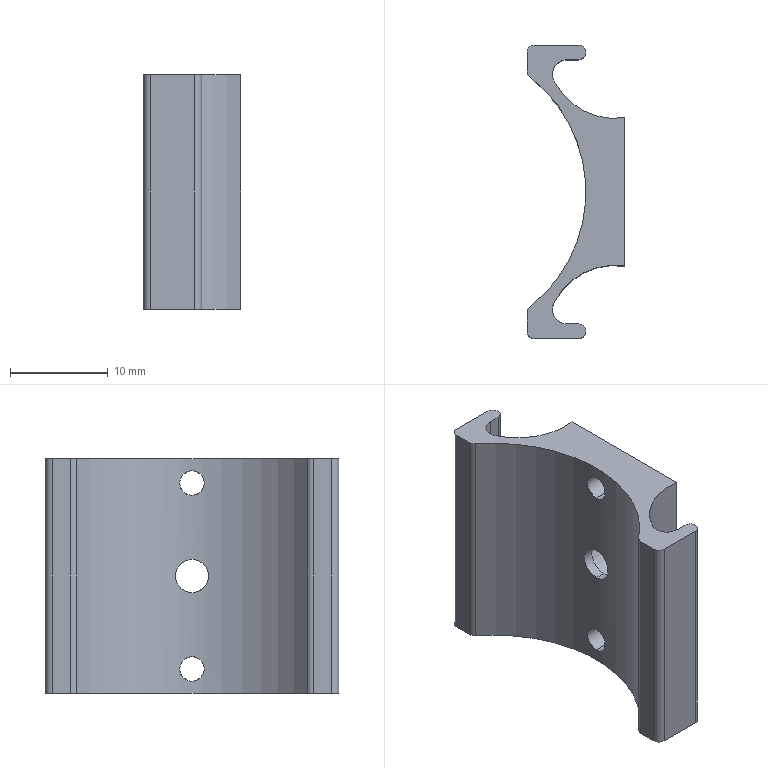Part | SolidWorks | features HoleWzd 2, Extrusion 1 | 1 solid | 31 faces | box 10 x 30 x 24 mm | volume 2596 mm3 | cylinder 21 | plane 10 | commonest cylinder face diameters 1.5 x6 2.5 x4 3 x4 3.4 x2 6 x2 14 x2
STEP:
#1=CARTESIAN_POINT('',(2.5,0.,3.));
#2=VERTEX_POINT('',#1);
#3=CARTESIAN_POINT('',(2.5,0.,-3.));
#4=VERTEX_POINT('',#3);
#5=CARTESIAN_POINT('',(2.5,0.,0.));
#6=DIRECTION('',(1.,0.,0.));
#7=DIRECTION('',(0.,0.,-1.));
#8=AXIS2_PLACEMENT_3D('',#5,#6,#7);
#9=CIRCLE('',#8,3.);
#10=EDGE_CURVE('',#2,#4,#9,.T.);
#11=ORIENTED_EDGE('',*,*,#10,.F.);
#12=CARTESIAN_POINT('',(5.5,0.,3.));
#13=VERTEX_POINT('',#12);
#14=CARTESIAN_POINT('',(5.5,0.,3.));
#15=DIRECTION('',(1.,0.,0.));
#16=VECTOR('',#15,1000.);
#17=LINE('',#14,#16);
#18=EDGE_CURVE('',#2,#13,#17,.T.);
#19=ORIENTED_EDGE('',*,*,#18,.T.);
#20=CARTESIAN_POINT('',(5.5,0.,-3.));
#21=VERTEX_POINT('',#20);
#22=CARTESIAN_POINT('',(5.5,0.,0.));
#23=DIRECTION('',(1.,0.,0.));
#24=DIRECTION('',(0.,0.,-1.));
#25=AXIS2_PLACEMENT_3D('',#22,#23,#24);
#26=CIRCLE('',#25,3.);
#27=EDGE_CURVE('',#13,#21,#26,.T.);
#28=ORIENTED_EDGE('',*,*,#27,.T.);
#29=CARTESIAN_POINT('',(5.5,0.,-3.));
#30=DIRECTION('',(1.,0.,0.));
#31=VECTOR('',#30,1000.);
#32=LINE('',#29,#31);
#33=EDGE_CURVE('',#4,#21,#32,.T.);
#34=ORIENTED_EDGE('',*,*,#33,.F.);
#35=EDGE_LOOP('',(#11,#19,#28,#34));
#36=FACE_OUTER_BOUND('',#35,.T.);
#37=CARTESIAN_POINT('',(5.5,0.,0.));
#38=DIRECTION('',(1.,0.,0.));
#39=DIRECTION('',(0.,0.,-1.));
#40=AXIS2_PLACEMENT_3D('',#37,#38,#39);
#41=CYLINDRICAL_SURFACE('',#40,3.);
#42=ADVANCED_FACE('',(#36),#41,.F.);
#43=CARTESIAN_POINT('',(1.5,0.,1.7));
#44=VERTEX_POINT('',#43);
#45=CARTESIAN_POINT('',(1.5,0.,-1.7));
#46=VERTEX_POINT('',#45);
#47=CARTESIAN_POINT('',(1.5,0.,1.7));
#48=CARTESIAN_POINT('',(1.5,-0.2219,1.7));
#49=CARTESIAN_POINT('',(1.495,-0.4457,1.655));
#50=CARTESIAN_POINT('',(1.477,-0.8549,1.486));
#51=CARTESIAN_POINT('',(1.464,-1.044,1.359));
#52=CARTESIAN_POINT('',(1.446,-1.28,1.125));
#53=CARTESIAN_POINT('',(1.439,-1.351,1.037));
#54=CARTESIAN_POINT('',(1.427,-1.475,0.8527));
#55=CARTESIAN_POINT('',(1.422,-1.527,0.7551));
#56=CARTESIAN_POINT('',(1.413,-1.613,0.5494));
#57=CARTESIAN_POINT('',(1.409,-1.645,0.4414));
#58=CARTESIAN_POINT('',(1.405,-1.689,0.2241));
#59=CARTESIAN_POINT('',(1.403,-1.7,0.1136));
#60=CARTESIAN_POINT('',(1.403,-1.7,-0.1111));
#61=CARTESIAN_POINT('',(1.405,-1.689,-0.2217));
#62=CARTESIAN_POINT('',(1.409,-1.646,-0.4391));
#63=CARTESIAN_POINT('',(1.413,-1.613,-0.5471));
#64=CARTESIAN_POINT('',(1.422,-1.528,-0.753));
#65=CARTESIAN_POINT('',(1.427,-1.476,-0.8506));
#66=CARTESIAN_POINT('',(1.439,-1.353,-1.035));
#67=CARTESIAN_POINT('',(1.445,-1.281,-1.123));
#68=CARTESIAN_POINT('',(1.464,-1.046,-1.358));
#69=CARTESIAN_POINT('',(1.477,-0.857,-1.485));
#70=CARTESIAN_POINT('',(1.495,-0.4481,-1.655));
#71=CARTESIAN_POINT('',(1.5,-0.2248,-1.7));
#72=CARTESIAN_POINT('',(1.5,0.,-1.7));
#73=B_SPLINE_CURVE_WITH_KNOTS('',3,(#47,#48,#49,#50,#51,#52,#53,#54,#55,#56,#57,#58,#59,#60,#61,#62,#63,#64,#65,#66,#67,#68,#69,#70,#71,#72),.UNSPECIFIED.,.F.,.F.,(4,2,2,2,2,2,2,2,2,2,2,2,4),(0.005319,0.005984,0.006649,0.006981,0.007313,0.007646,0.007978,0.008311,0.008643,0.008975,0.009308,0.009972,0.01064),.UNSPECIFIED.);
#74=EDGE_CURVE('',#44,#46,#73,.T.);
#75=ORIENTED_EDGE('',*,*,#74,.F.);
#76=CARTESIAN_POINT('',(2.5,0.,1.7));
#77=VERTEX_POINT('',#76);
#78=CARTESIAN_POINT('',(5.5,0.,1.7));
#79=DIRECTION('',(1.,0.,0.));
#80=VECTOR('',#79,1000.);
#81=LINE('',#78,#80);
#82=EDGE_CURVE('',#44,#77,#81,.T.);
#83=ORIENTED_EDGE('',*,*,#82,.T.);
#84=CARTESIAN_POINT('',(2.5,0.,-1.7));
#85=VERTEX_POINT('',#84);
#86=CARTESIAN_POINT('',(2.5,0.,0.));
#87=DIRECTION('',(1.,0.,0.));
#88=DIRECTION('',(0.,0.,-1.));
#89=AXIS2_PLACEMENT_3D('',#86,#87,#88);
#90=CIRCLE('',#89,1.7);
#91=EDGE_CURVE('',#77,#85,#90,.T.);
#92=ORIENTED_EDGE('',*,*,#91,.T.);
#93=CARTESIAN_POINT('',(5.5,0.,-1.7));
#94=DIRECTION('',(1.,0.,0.));
#95=VECTOR('',#94,1000.);
#96=LINE('',#93,#95);
#97=EDGE_CURVE('',#46,#85,#96,.T.);
#98=ORIENTED_EDGE('',*,*,#97,.F.);
#99=EDGE_LOOP('',(#75,#83,#92,#98));
#100=FACE_OUTER_BOUND('',#99,.T.);
#101=CARTESIAN_POINT('',(5.5,0.,0.));
#102=DIRECTION('',(1.,0.,0.));
#103=DIRECTION('',(0.,0.,-1.));
#104=AXIS2_PLACEMENT_3D('',#101,#102,#103);
#105=CYLINDRICAL_SURFACE('',#104,1.7);
#106=ADVANCED_FACE('',(#100),#105,.F.);
#107=CARTESIAN_POINT('',(1.5,0.,10.75));
#108=VERTEX_POINT('',#107);
#109=CARTESIAN_POINT('',(1.5,0.,8.25));
#110=VERTEX_POINT('',#109);
#111=CARTESIAN_POINT('',(1.5,0.,10.75));
#112=CARTESIAN_POINT('',(1.5,-0.1632,10.75));
#113=CARTESIAN_POINT('',(1.497,-0.3276,10.717));
#114=CARTESIAN_POINT('',(1.488,-0.6285,10.593));
#115=CARTESIAN_POINT('',(1.481,-0.768,10.5));
#116=CARTESIAN_POINT('',(1.467,-0.9986,10.269));
#117=CARTESIAN_POINT('',(1.46,-1.092,10.131));
#118=CARTESIAN_POINT('',(1.451,-1.217,9.828));
#119=CARTESIAN_POINT('',(1.448,-1.25,9.666));
#120=CARTESIAN_POINT('',(1.448,-1.25,9.336));
#121=CARTESIAN_POINT('',(1.451,-1.218,9.174));
#122=CARTESIAN_POINT('',(1.458,-1.124,8.946));
#123=CARTESIAN_POINT('',(1.461,-1.085,8.875));
#124=CARTESIAN_POINT('',(1.467,-0.9948,8.739));
#125=CARTESIAN_POINT('',(1.47,-0.9421,8.674));
#126=CARTESIAN_POINT('',(1.481,-0.7693,8.501));
#127=CARTESIAN_POINT('',(1.488,-0.63,8.408));
#128=CARTESIAN_POINT('',(1.497,-0.3294,8.283));
#129=CARTESIAN_POINT('',(1.5,-0.1652,8.25));
#130=CARTESIAN_POINT('',(1.5,0.,8.25));
#131=B_SPLINE_CURVE_WITH_KNOTS('',3,(#111,#112,#113,#114,#115,#116,#117,#118,#119,#120,#121,#122,#123,#124,#125,#126,#127,#128,#129,#130),.UNSPECIFIED.,.F.,.F.,(4,2,2,2,2,2,2,2,2,4),(0.00391,0.004398,0.004887,0.005376,0.005864,0.006353,0.006597,0.006841,0.00733,0.007819),.UNSPECIFIED.);
#132=EDGE_CURVE('',#108,#110,#131,.T.);
#133=ORIENTED_EDGE('',*,*,#132,.F.);
#134=CARTESIAN_POINT('',(5.5,0.,10.75));
#135=VERTEX_POINT('',#134);
#136=CARTESIAN_POINT('',(5.5,0.,10.75));
#137=DIRECTION('',(1.,0.,0.));
#138=VECTOR('',#137,1000.);
#139=LINE('',#136,#138);
#140=EDGE_CURVE('',#108,#135,#139,.T.);
#141=ORIENTED_EDGE('',*,*,#140,.T.);
#142=CARTESIAN_POINT('',(5.5,0.,8.25));
#143=VERTEX_POINT('',#142);
#144=CARTESIAN_POINT('',(5.5,0.,9.5));
#145=DIRECTION('',(1.,0.,0.));
#146=DIRECTION('',(0.,0.,-1.));
#147=AXIS2_PLACEMENT_3D('',#144,#145,#146);
#148=CIRCLE('',#147,1.25);
#149=EDGE_CURVE('',#135,#143,#148,.T.);
#150=ORIENTED_EDGE('',*,*,#149,.T.);
#151=CARTESIAN_POINT('',(5.5,0.,8.25));
#152=DIRECTION('',(1.,0.,0.));
#153=VECTOR('',#152,1000.);
#154=LINE('',#151,#153);
#155=EDGE_CURVE('',#110,#143,#154,.T.);
#156=ORIENTED_EDGE('',*,*,#155,.F.);
#157=EDGE_LOOP('',(#133,#141,#150,#156));
#158=FACE_OUTER_BOUND('',#157,.T.);
#159=CARTESIAN_POINT('',(5.5,0.,9.5));
#160=DIRECTION('',(1.,0.,0.));
#161=DIRECTION('',(0.,0.,-1.));
#162=AXIS2_PLACEMENT_3D('',#159,#160,#161);
#163=CYLINDRICAL_SURFACE('',#162,1.25);
#164=ADVANCED_FACE('',(#158),#163,.F.);
#165=CARTESIAN_POINT('',(1.5,0.,-8.25));
#166=VERTEX_POINT('',#165);
#167=CARTESIAN_POINT('',(1.5,0.,-10.75));
#168=VERTEX_POINT('',#167);
#169=CARTESIAN_POINT('',(1.5,0.,-8.25));
#170=CARTESIAN_POINT('',(1.5,-0.1632,-8.25));
#171=CARTESIAN_POINT('',(1.497,-0.3276,-8.283));
#172=CARTESIAN_POINT('',(1.488,-0.6285,-8.407));
#173=CARTESIAN_POINT('',(1.481,-0.768,-8.5));
#174=CARTESIAN_POINT('',(1.467,-0.9986,-8.731));
#175=CARTESIAN_POINT('',(1.46,-1.092,-8.869));
#176=CARTESIAN_POINT('',(1.451,-1.217,-9.172));
#177=CARTESIAN_POINT('',(1.448,-1.25,-9.334));
#178=CARTESIAN_POINT('',(1.448,-1.25,-9.664));
#179=CARTESIAN_POINT('',(1.451,-1.218,-9.826));
#180=CARTESIAN_POINT('',(1.458,-1.124,-10.054));
#181=CARTESIAN_POINT('',(1.461,-1.085,-10.125));
#182=CARTESIAN_POINT('',(1.467,-0.9948,-10.261));
#183=CARTESIAN_POINT('',(1.47,-0.9421,-10.326));
#184=CARTESIAN_POINT('',(1.481,-0.7693,-10.499));
#185=CARTESIAN_POINT('',(1.488,-0.63,-10.592));
#186=CARTESIAN_POINT('',(1.497,-0.3294,-10.717));
#187=CARTESIAN_POINT('',(1.5,-0.1652,-10.75));
#188=CARTESIAN_POINT('',(1.5,0.,-10.75));
#189=B_SPLINE_CURVE_WITH_KNOTS('',3,(#169,#170,#171,#172,#173,#174,#175,#176,#177,#178,#179,#180,#181,#182,#183,#184,#185,#186,#187,#188),.UNSPECIFIED.,.F.,.F.,(4,2,2,2,2,2,2,2,2,4),(0.00391,0.004398,0.004887,0.005376,0.005864,0.006353,0.006597,0.006841,0.00733,0.007819),.UNSPECIFIED.);
#190=EDGE_CURVE('',#166,#168,#189,.T.);
#191=ORIENTED_EDGE('',*,*,#190,.F.);
#192=CARTESIAN_POINT('',(5.5,0.,-8.25));
#193=VERTEX_POINT('',#192);
#194=CARTESIAN_POINT('',(5.5,0.,-8.25));
#195=DIRECTION('',(1.,0.,0.));
#196=VECTOR('',#195,1000.);
#197=LINE('',#194,#196);
#198=EDGE_CURVE('',#166,#193,#197,.T.);
#199=ORIENTED_EDGE('',*,*,#198,.T.);
#200=CARTESIAN_POINT('',(5.5,0.,-10.75));
#201=VERTEX_POINT('',#200);
#202=CARTESIAN_POINT('',(5.5,0.,-9.5));
#203=DIRECTION('',(1.,0.,0.));
#204=DIRECTION('',(0.,0.,-1.));
#205=AXIS2_PLACEMENT_3D('',#202,#203,#204);
#206=CIRCLE('',#205,1.25);
#207=EDGE_CURVE('',#193,#201,#206,.T.);
#208=ORIENTED_EDGE('',*,*,#207,.T.);
#209=CARTESIAN_POINT('',(5.5,0.,-10.75));
#210=DIRECTION('',(1.,0.,0.));
#211=VECTOR('',#210,1000.);
#212=LINE('',#209,#211);
#213=EDGE_CURVE('',#168,#201,#212,.T.);
#214=ORIENTED_EDGE('',*,*,#213,.F.);
#215=EDGE_LOOP('',(#191,#199,#208,#214));
#216=FACE_OUTER_BOUND('',#215,.T.);
#217=CARTESIAN_POINT('',(5.5,0.,-9.5));
#218=DIRECTION('',(1.,0.,0.));
#219=DIRECTION('',(0.,0.,-1.));
#220=AXIS2_PLACEMENT_3D('',#217,#218,#219);
#221=CYLINDRICAL_SURFACE('',#220,1.25);
#222=ADVANCED_FACE('',(#216),#221,.F.);
#223=CARTESIAN_POINT('',(-1.899,-12.,12.));
#224=VERTEX_POINT('',#223);
#225=CARTESIAN_POINT('',(-1.735,-11.318,12.));
#226=VERTEX_POINT('',#225);
#227=CARTESIAN_POINT('',(-0.399,-12.,12.));
#228=DIRECTION('',(0.,0.,-1.));
#229=DIRECTION('',(1.,0.,0.));
#230=AXIS2_PLACEMENT_3D('',#227,#228,#229);
#231=CIRCLE('',#230,1.5);
#232=EDGE_CURVE('',#224,#226,#231,.T.);
#233=ORIENTED_EDGE('',*,*,#232,.F.);
#234=CARTESIAN_POINT('',(-1.899,-12.,-12.));
#235=VERTEX_POINT('',#234);
#236=CARTESIAN_POINT('',(-1.899,-12.,12.));
#237=DIRECTION('',(0.,0.,-1.));
#238=VECTOR('',#237,1000.);
#239=LINE('',#236,#238);
#240=EDGE_CURVE('',#224,#235,#239,.T.);
#241=ORIENTED_EDGE('',*,*,#240,.T.);
#242=CARTESIAN_POINT('',(-1.735,-11.318,-12.));
#243=VERTEX_POINT('',#242);
#244=CARTESIAN_POINT('',(-0.399,-12.,-12.));
#245=DIRECTION('',(0.,0.,-1.));
#246=DIRECTION('',(1.,0.,0.));
#247=AXIS2_PLACEMENT_3D('',#244,#245,#246);
#248=CIRCLE('',#247,1.5);
#249=EDGE_CURVE('',#235,#243,#248,.T.);
#250=ORIENTED_EDGE('',*,*,#249,.T.);
#251=CARTESIAN_POINT('',(-1.735,-11.318,12.));
#252=DIRECTION('',(0.,0.,-1.));
#253=VECTOR('',#252,1000.);
#254=LINE('',#251,#253);
#255=EDGE_CURVE('',#226,#243,#254,.T.);
#256=ORIENTED_EDGE('',*,*,#255,.F.);
#257=EDGE_LOOP('',(#233,#241,#250,#256));
#258=FACE_OUTER_BOUND('',#257,.T.);
#259=CARTESIAN_POINT('',(-0.399,-12.,12.));
#260=DIRECTION('',(0.,0.,-1.));
#261=DIRECTION('',(-1.,0.,0.));
#262=AXIS2_PLACEMENT_3D('',#259,#260,#261);
#263=CYLINDRICAL_SURFACE('',#262,1.5);
#264=ADVANCED_FACE('',(#258),#263,.F.);
#265=CARTESIAN_POINT('',(-1.899,12.,12.));
#266=VERTEX_POINT('',#265);
#267=CARTESIAN_POINT('',(-0.399,13.5,12.));
#268=VERTEX_POINT('',#267);
#269=CARTESIAN_POINT('',(-0.399,12.,12.));
#270=DIRECTION('',(0.,0.,-1.));
#271=DIRECTION('',(1.,0.,0.));
#272=AXIS2_PLACEMENT_3D('',#269,#270,#271);
#273=CIRCLE('',#272,1.5);
#274=EDGE_CURVE('',#266,#268,#273,.T.);
#275=ORIENTED_EDGE('',*,*,#274,.F.);
#276=CARTESIAN_POINT('',(-1.899,12.,-12.));
#277=VERTEX_POINT('',#276);
#278=CARTESIAN_POINT('',(-1.899,12.,12.));
#279=DIRECTION('',(0.,0.,-1.));
#280=VECTOR('',#279,1000.);
#281=LINE('',#278,#280);
#282=EDGE_CURVE('',#266,#277,#281,.T.);
#283=ORIENTED_EDGE('',*,*,#282,.T.);
#284=CARTESIAN_POINT('',(-0.399,13.5,-12.));
#285=VERTEX_POINT('',#284);
#286=CARTESIAN_POINT('',(-0.399,12.,-12.));
#287=DIRECTION('',(0.,0.,-1.));
#288=DIRECTION('',(1.,0.,0.));
#289=AXIS2_PLACEMENT_3D('',#286,#287,#288);
#290=CIRCLE('',#289,1.5);
#291=EDGE_CURVE('',#277,#285,#290,.T.);
#292=ORIENTED_EDGE('',*,*,#291,.T.);
#293=CARTESIAN_POINT('',(-0.399,13.5,12.));
#294=DIRECTION('',(0.,0.,-1.));
#295=VECTOR('',#294,1000.);
#296=LINE('',#293,#295);
#297=EDGE_CURVE('',#268,#285,#296,.T.);
#298=ORIENTED_EDGE('',*,*,#297,.F.);
#299=EDGE_LOOP('',(#275,#283,#292,#298));
#300=FACE_OUTER_BOUND('',#299,.T.);
#301=CARTESIAN_POINT('',(-0.399,12.,12.));
#302=DIRECTION('',(0.,0.,-1.));
#303=DIRECTION('',(-1.,0.,0.));
#304=AXIS2_PLACEMENT_3D('',#301,#302,#303);
#305=CYLINDRICAL_SURFACE('',#304,1.5);
#306=ADVANCED_FACE('',(#300),#305,.F.);
#307=ORIENTED_EDGE('',*,*,#282,.F.);
#308=CARTESIAN_POINT('',(-1.735,11.318,12.));
#309=VERTEX_POINT('',#308);
#310=CARTESIAN_POINT('',(-0.399,12.,12.));
#311=DIRECTION('',(0.,0.,-1.));
#312=DIRECTION('',(1.,0.,0.));
#313=AXIS2_PLACEMENT_3D('',#310,#311,#312);
#314=CIRCLE('',#313,1.5);
#315=EDGE_CURVE('',#309,#266,#314,.T.);
#316=ORIENTED_EDGE('',*,*,#315,.F.);
#317=CARTESIAN_POINT('',(-1.735,11.318,-12.));
#318=VERTEX_POINT('',#317);
#319=CARTESIAN_POINT('',(-1.735,11.318,12.));
#320=DIRECTION('',(0.,0.,-1.));
#321=VECTOR('',#320,1000.);
#322=LINE('',#319,#321);
#323=EDGE_CURVE('',#309,#318,#322,.T.);
#324=ORIENTED_EDGE('',*,*,#323,.T.);
#325=CARTESIAN_POINT('',(-0.399,12.,-12.));
#326=DIRECTION('',(0.,0.,-1.));
#327=DIRECTION('',(1.,0.,0.));
#328=AXIS2_PLACEMENT_3D('',#325,#326,#327);
#329=CIRCLE('',#328,1.5);
#330=EDGE_CURVE('',#318,#277,#329,.T.);
#331=ORIENTED_EDGE('',*,*,#330,.T.);
#332=EDGE_LOOP('',(#307,#316,#324,#331));
#333=FACE_OUTER_BOUND('',#332,.T.);
#334=CARTESIAN_POINT('',(-0.399,12.,12.));
#335=DIRECTION('',(0.,0.,-1.));
#336=DIRECTION('',(-1.,0.,0.));
#337=AXIS2_PLACEMENT_3D('',#334,#335,#336);
#338=CYLINDRICAL_SURFACE('',#337,1.5);
#339=ADVANCED_FACE('',(#333),#338,.F.);
#340=CARTESIAN_POINT('',(0.75,13.5,-12.));
#341=VERTEX_POINT('',#340);
#342=CARTESIAN_POINT('',(-0.399,13.5,-12.));
#343=DIRECTION('',(1.,0.,0.));
#344=VECTOR('',#343,1000.);
#345=LINE('',#342,#344);
#346=EDGE_CURVE('',#285,#341,#345,.T.);
#347=ORIENTED_EDGE('',*,*,#346,.T.);
#348=CARTESIAN_POINT('',(0.75,13.5,12.));
#349=VERTEX_POINT('',#348);
#350=CARTESIAN_POINT('',(0.75,13.5,12.));
#351=DIRECTION('',(0.,0.,-1.));
#352=VECTOR('',#351,1000.);
#353=LINE('',#350,#352);
#354=EDGE_CURVE('',#349,#341,#353,.T.);
#355=ORIENTED_EDGE('',*,*,#354,.F.);
#356=CARTESIAN_POINT('',(-0.399,13.5,12.));
#357=DIRECTION('',(1.,0.,0.));
#358=VECTOR('',#357,1000.);
#359=LINE('',#356,#358);
#360=EDGE_CURVE('',#268,#349,#359,.T.);
#361=ORIENTED_EDGE('',*,*,#360,.F.);
#362=ORIENTED_EDGE('',*,*,#297,.T.);
#363=EDGE_LOOP('',(#347,#355,#361,#362));
#364=FACE_OUTER_BOUND('',#363,.T.);
#365=CARTESIAN_POINT('',(-0.399,13.5,12.));
#366=DIRECTION('',(0.,1.,0.));
#367=DIRECTION('',(0.,0.,1.));
#368=AXIS2_PLACEMENT_3D('',#365,#366,#367);
#369=PLANE('',#368);
#370=ADVANCED_FACE('',(#364),#369,.F.);
#371=CARTESIAN_POINT('',(0.75,15.,-12.));
#372=VERTEX_POINT('',#371);
#373=CARTESIAN_POINT('',(0.75,14.25,-12.));
#374=DIRECTION('',(0.,0.,1.));
#375=DIRECTION('',(1.,0.,0.));
#376=AXIS2_PLACEMENT_3D('',#373,#374,#375);
#377=CIRCLE('',#376,0.75);
#378=EDGE_CURVE('',#341,#372,#377,.T.);
#379=ORIENTED_EDGE('',*,*,#378,.T.);
#380=CARTESIAN_POINT('',(0.75,15.,12.));
#381=VERTEX_POINT('',#380);
#382=CARTESIAN_POINT('',(0.75,15.,12.));
#383=DIRECTION('',(0.,0.,-1.));
#384=VECTOR('',#383,1000.);
#385=LINE('',#382,#384);
#386=EDGE_CURVE('',#381,#372,#385,.T.);
#387=ORIENTED_EDGE('',*,*,#386,.F.);
#388=CARTESIAN_POINT('',(0.75,14.25,12.));
#389=DIRECTION('',(0.,0.,1.));
#390=DIRECTION('',(1.,0.,0.));
#391=AXIS2_PLACEMENT_3D('',#388,#389,#390);
#392=CIRCLE('',#391,0.75);
#393=EDGE_CURVE('',#349,#381,#392,.T.);
#394=ORIENTED_EDGE('',*,*,#393,.F.);
#395=ORIENTED_EDGE('',*,*,#354,.T.);
#396=EDGE_LOOP('',(#379,#387,#394,#395));
#397=FACE_OUTER_BOUND('',#396,.T.);
#398=CARTESIAN_POINT('',(0.75,14.25,12.));
#399=DIRECTION('',(0.,0.,-1.));
#400=DIRECTION('',(-1.,0.,0.));
#401=AXIS2_PLACEMENT_3D('',#398,#399,#400);
#402=CYLINDRICAL_SURFACE('',#401,0.75);
#403=ADVANCED_FACE('',(#397),#402,.T.);
#404=CARTESIAN_POINT('',(-3.75,15.,-12.));
#405=VERTEX_POINT('',#404);
#406=CARTESIAN_POINT('',(0.75,15.,-12.));
#407=DIRECTION('',(-1.,0.,0.));
#408=VECTOR('',#407,1000.);
#409=LINE('',#406,#408);
#410=EDGE_CURVE('',#372,#405,#409,.T.);
#411=ORIENTED_EDGE('',*,*,#410,.T.);
#412=CARTESIAN_POINT('',(-3.75,15.,12.));
#413=VERTEX_POINT('',#412);
#414=CARTESIAN_POINT('',(-3.75,15.,12.));
#415=DIRECTION('',(0.,0.,-1.));
#416=VECTOR('',#415,1000.);
#417=LINE('',#414,#416);
#418=EDGE_CURVE('',#413,#405,#417,.T.);
#419=ORIENTED_EDGE('',*,*,#418,.F.);
#420=CARTESIAN_POINT('',(0.75,15.,12.));
#421=DIRECTION('',(-1.,0.,0.));
#422=VECTOR('',#421,1000.);
#423=LINE('',#420,#422);
#424=EDGE_CURVE('',#381,#413,#423,.T.);
#425=ORIENTED_EDGE('',*,*,#424,.F.);
#426=ORIENTED_EDGE('',*,*,#386,.T.);
#427=EDGE_LOOP('',(#411,#419,#425,#426));
#428=FACE_OUTER_BOUND('',#427,.T.);
#429=CARTESIAN_POINT('',(0.75,15.,12.));
#430=DIRECTION('',(0.,-1.,0.));
#431=DIRECTION('',(1.,0.,0.));
#432=AXIS2_PLACEMENT_3D('',#429,#430,#431);
#433=PLANE('',#432);
#434=ADVANCED_FACE('',(#428),#433,.F.);
#435=CARTESIAN_POINT('',(-4.5,14.25,-12.));
#436=VERTEX_POINT('',#435);
#437=CARTESIAN_POINT('',(-3.75,14.25,-12.));
#438=DIRECTION('',(0.,0.,1.));
#439=DIRECTION('',(1.,0.,0.));
#440=AXIS2_PLACEMENT_3D('',#437,#438,#439);
#441=CIRCLE('',#440,0.75);
#442=EDGE_CURVE('',#405,#436,#441,.T.);
#443=ORIENTED_EDGE('',*,*,#442,.T.);
#444=CARTESIAN_POINT('',(-4.5,14.25,12.));
#445=VERTEX_POINT('',#444);
#446=CARTESIAN_POINT('',(-4.5,14.25,12.));
#447=DIRECTION('',(0.,0.,-1.));
#448=VECTOR('',#447,1000.);
#449=LINE('',#446,#448);
#450=EDGE_CURVE('',#445,#436,#449,.T.);
#451=ORIENTED_EDGE('',*,*,#450,.F.);
#452=CARTESIAN_POINT('',(-3.75,14.25,12.));
#453=DIRECTION('',(0.,0.,1.));
#454=DIRECTION('',(1.,0.,0.));
#455=AXIS2_PLACEMENT_3D('',#452,#453,#454);
#456=CIRCLE('',#455,0.75);
#457=EDGE_CURVE('',#413,#445,#456,.T.);
#458=ORIENTED_EDGE('',*,*,#457,.F.);
#459=ORIENTED_EDGE('',*,*,#418,.T.);
#460=EDGE_LOOP('',(#443,#451,#458,#459));
#461=FACE_OUTER_BOUND('',#460,.T.);
#462=CARTESIAN_POINT('',(-3.75,14.25,12.));
#463=DIRECTION('',(0.,0.,-1.));
#464=DIRECTION('',(-1.,0.,0.));
#465=AXIS2_PLACEMENT_3D('',#462,#463,#464);
#466=CYLINDRICAL_SURFACE('',#465,0.75);
#467=ADVANCED_FACE('',(#461),#466,.T.);
#468=CARTESIAN_POINT('',(-4.5,12.369,-12.));
#469=VERTEX_POINT('',#468);
#470=CARTESIAN_POINT('',(-4.5,14.25,-12.));
#471=DIRECTION('',(0.,-1.,0.));
#472=VECTOR('',#471,1000.);
#473=LINE('',#470,#472);
#474=EDGE_CURVE('',#436,#469,#473,.T.);
#475=ORIENTED_EDGE('',*,*,#474,.T.);
#476=CARTESIAN_POINT('',(-4.5,12.369,12.));
#477=VERTEX_POINT('',#476);
#478=CARTESIAN_POINT('',(-4.5,12.369,12.));
#479=DIRECTION('',(0.,0.,-1.));
#480=VECTOR('',#479,1000.);
#481=LINE('',#478,#480);
#482=EDGE_CURVE('',#477,#469,#481,.T.);
#483=ORIENTED_EDGE('',*,*,#482,.F.);
#484=CARTESIAN_POINT('',(-4.5,14.25,12.));
#485=DIRECTION('',(0.,-1.,0.));
#486=VECTOR('',#485,1000.);
#487=LINE('',#484,#486);
#488=EDGE_CURVE('',#445,#477,#487,.T.);
#489=ORIENTED_EDGE('',*,*,#488,.F.);
#490=ORIENTED_EDGE('',*,*,#450,.T.);
#491=EDGE_LOOP('',(#475,#483,#489,#490));
#492=FACE_OUTER_BOUND('',#491,.T.);
#493=CARTESIAN_POINT('',(-4.5,14.25,12.));
#494=DIRECTION('',(1.,0.,0.));
#495=DIRECTION('',(0.,0.,-1.));
#496=AXIS2_PLACEMENT_3D('',#493,#494,#495);
#497=PLANE('',#496);
#498=ADVANCED_FACE('',(#492),#497,.F.);
#499=CARTESIAN_POINT('',(-4.214,11.78,-12.));
#500=VERTEX_POINT('',#499);
#501=CARTESIAN_POINT('',(-3.75,12.369,-12.));
#502=DIRECTION('',(0.,0.,1.));
#503=DIRECTION('',(1.,0.,0.));
#504=AXIS2_PLACEMENT_3D('',#501,#502,#503);
#505=CIRCLE('',#504,0.75);
#506=EDGE_CURVE('',#469,#500,#505,.T.);
#507=ORIENTED_EDGE('',*,*,#506,.T.);
#508=CARTESIAN_POINT('',(-4.214,11.78,12.));
#509=VERTEX_POINT('',#508);
#510=CARTESIAN_POINT('',(-4.214,11.78,12.));
#511=DIRECTION('',(0.,0.,-1.));
#512=VECTOR('',#511,1000.);
#513=LINE('',#510,#512);
#514=EDGE_CURVE('',#509,#500,#513,.T.);
#515=ORIENTED_EDGE('',*,*,#514,.F.);
#516=CARTESIAN_POINT('',(-3.75,12.369,12.));
#517=DIRECTION('',(0.,0.,1.));
#518=DIRECTION('',(1.,0.,0.));
#519=AXIS2_PLACEMENT_3D('',#516,#517,#518);
#520=CIRCLE('',#519,0.75);
#521=EDGE_CURVE('',#477,#509,#520,.T.);
#522=ORIENTED_EDGE('',*,*,#521,.F.);
#523=ORIENTED_EDGE('',*,*,#482,.T.);
#524=EDGE_LOOP('',(#507,#515,#522,#523));
#525=FACE_OUTER_BOUND('',#524,.T.);
#526=CARTESIAN_POINT('',(-3.75,12.369,12.));
#527=DIRECTION('',(0.,0.,-1.));
#528=DIRECTION('',(-1.,0.,0.));
#529=AXIS2_PLACEMENT_3D('',#526,#527,#528);
#530=CYLINDRICAL_SURFACE('',#529,0.75);
#531=ADVANCED_FACE('',(#525),#530,.T.);
#532=CARTESIAN_POINT('',(1.5,0.,-1.7));
#533=CARTESIAN_POINT('',(1.5,0.1124,-1.7));
#534=CARTESIAN_POINT('',(1.499,0.2229,-1.689));
#535=CARTESIAN_POINT('',(1.494,0.4404,-1.646));
#536=CARTESIAN_POINT('',(1.49,0.5484,-1.613));
#537=CARTESIAN_POINT('',(1.481,0.7542,-1.528));
#538=CARTESIAN_POINT('',(1.476,0.8518,-1.475));
#539=CARTESIAN_POINT('',(1.464,1.037,-1.352));
#540=CARTESIAN_POINT('',(1.458,1.124,-1.28));
#541=CARTESIAN_POINT('',(1.439,1.359,-1.045));
#542=CARTESIAN_POINT('',(1.426,1.486,-0.8555));
#543=CARTESIAN_POINT('',(1.409,1.655,-0.4464));
#544=CARTESIAN_POINT('',(1.403,1.7,-0.2226));
#545=CARTESIAN_POINT('',(1.403,1.7,0.1104));
#546=CARTESIAN_POINT('',(1.405,1.689,0.2231));
#547=CARTESIAN_POINT('',(1.409,1.646,0.4412));
#548=CARTESIAN_POINT('',(1.413,1.613,0.5472));
#549=CARTESIAN_POINT('',(1.422,1.528,0.7532));
#550=CARTESIAN_POINT('',(1.427,1.475,0.8526));
#551=CARTESIAN_POINT('',(1.439,1.352,1.037));
#552=CARTESIAN_POINT('',(1.445,1.282,1.123));
#553=CARTESIAN_POINT('',(1.458,1.123,1.281));
#554=CARTESIAN_POINT('',(1.464,1.037,1.352));
#555=CARTESIAN_POINT('',(1.476,0.8531,1.475));
#556=CARTESIAN_POINT('',(1.481,0.7536,1.528));
#557=CARTESIAN_POINT('',(1.49,0.5478,1.613));
#558=CARTESIAN_POINT('',(1.494,0.4418,1.645));
#559=CARTESIAN_POINT('',(1.499,0.2237,1.689));
#560=CARTESIAN_POINT('',(1.5,0.111,1.7));
#561=CARTESIAN_POINT('',(1.5,0.,1.7));
#562=B_SPLINE_CURVE_WITH_KNOTS('',3,(#532,#533,#534,#535,#536,#537,#538,#539,#540,#541,#542,#543,#544,#545,#546,#547,#548,#549,#550,#551,#552,#553,#554,#555,#556,#557,#558,#559,#560,#561),.UNSPECIFIED.,.F.,.F.,(4,2,2,2,2,2,2,2,2,2,2,2,2,2,4),(0.,0.0003325,0.0006649,0.0009974,0.00133,0.001995,0.00266,0.002992,0.003325,0.003657,0.003989,0.004322,0.004654,0.004987,0.005319),.UNSPECIFIED.);
#563=EDGE_CURVE('',#46,#44,#562,.T.);
#564=ORIENTED_EDGE('',*,*,#563,.T.);
#565=ORIENTED_EDGE('',*,*,#74,.T.);
#566=EDGE_LOOP('',(#564,#565));
#567=FACE_BOUND('',#566,.T.);
#568=CARTESIAN_POINT('',(1.5,0.,8.25));
#569=CARTESIAN_POINT('',(1.5,0.1653,8.25));
#570=CARTESIAN_POINT('',(1.497,0.3274,8.283));
#571=CARTESIAN_POINT('',(1.488,0.6302,8.408));
#572=CARTESIAN_POINT('',(1.481,0.7688,8.501));
#573=CARTESIAN_POINT('',(1.467,0.9993,8.732));
#574=CARTESIAN_POINT('',(1.46,1.092,8.871));
#575=CARTESIAN_POINT('',(1.451,1.217,9.172));
#576=CARTESIAN_POINT('',(1.448,1.25,9.336));
#577=CARTESIAN_POINT('',(1.448,1.25,9.663));
#578=CARTESIAN_POINT('',(1.451,1.218,9.827));
#579=CARTESIAN_POINT('',(1.46,1.092,10.129));
#580=CARTESIAN_POINT('',(1.467,1.001,10.267));
#581=CARTESIAN_POINT('',(1.481,0.7674,10.5));
#582=CARTESIAN_POINT('',(1.488,0.6298,10.592));
#583=CARTESIAN_POINT('',(1.495,0.4027,10.686));
#584=CARTESIAN_POINT('',(1.497,0.3247,10.71));
#585=CARTESIAN_POINT('',(1.499,0.1645,10.742));
#586=CARTESIAN_POINT('',(1.5,0.0816,10.75));
#587=CARTESIAN_POINT('',(1.5,0.,10.75));
#588=B_SPLINE_CURVE_WITH_KNOTS('',3,(#568,#569,#570,#571,#572,#573,#574,#575,#576,#577,#578,#579,#580,#581,#582,#583,#584,#585,#586,#587),.UNSPECIFIED.,.F.,.F.,(4,2,2,2,2,2,2,2,2,4),(0.,0.0004887,0.0009774,0.001466,0.001955,0.002444,0.002932,0.003421,0.003665,0.00391),.UNSPECIFIED.);
#589=EDGE_CURVE('',#110,#108,#588,.T.);
#590=ORIENTED_EDGE('',*,*,#589,.T.);
#591=ORIENTED_EDGE('',*,*,#132,.T.);
#592=EDGE_LOOP('',(#590,#591));
#593=FACE_BOUND('',#592,.T.);
#594=CARTESIAN_POINT('',(1.5,0.,-10.75));
#595=CARTESIAN_POINT('',(1.5,0.1653,-10.75));
#596=CARTESIAN_POINT('',(1.497,0.3274,-10.717));
#597=CARTESIAN_POINT('',(1.488,0.6302,-10.592));
#598=CARTESIAN_POINT('',(1.481,0.7688,-10.499));
#599=CARTESIAN_POINT('',(1.467,0.9993,-10.268));
#600=CARTESIAN_POINT('',(1.46,1.092,-10.129));
#601=CARTESIAN_POINT('',(1.451,1.217,-9.828));
#602=CARTESIAN_POINT('',(1.448,1.25,-9.664));
#603=CARTESIAN_POINT('',(1.448,1.25,-9.337));
#604=CARTESIAN_POINT('',(1.451,1.218,-9.173));
#605=CARTESIAN_POINT('',(1.46,1.092,-8.871));
#606=CARTESIAN_POINT('',(1.467,1.001,-8.733));
#607=CARTESIAN_POINT('',(1.481,0.7674,-8.5));
#608=CARTESIAN_POINT('',(1.488,0.6298,-8.408));
#609=CARTESIAN_POINT('',(1.495,0.4027,-8.314));
#610=CARTESIAN_POINT('',(1.497,0.3247,-8.29));
#611=CARTESIAN_POINT('',(1.499,0.1645,-8.258));
#612=CARTESIAN_POINT('',(1.5,0.0816,-8.25));
#613=CARTESIAN_POINT('',(1.5,0.,-8.25));
#614=B_SPLINE_CURVE_WITH_KNOTS('',3,(#594,#595,#596,#597,#598,#599,#600,#601,#602,#603,#604,#605,#606,#607,#608,#609,#610,#611,#612,#613),.UNSPECIFIED.,.F.,.F.,(4,2,2,2,2,2,2,2,2,4),(0.,0.0004887,0.0009774,0.001466,0.001955,0.002444,0.002932,0.003421,0.003665,0.00391),.UNSPECIFIED.);
#615=EDGE_CURVE('',#168,#166,#614,.T.);
#616=ORIENTED_EDGE('',*,*,#615,.T.);
#617=ORIENTED_EDGE('',*,*,#190,.T.);
#618=EDGE_LOOP('',(#616,#617));
#619=FACE_BOUND('',#618,.T.);
#620=CARTESIAN_POINT('',(-4.214,-11.78,-12.));
#621=VERTEX_POINT('',#620);
#622=CARTESIAN_POINT('',(-13.5,0.,-12.));
#623=DIRECTION('',(0.,0.,-1.));
#624=DIRECTION('',(1.,0.,0.));
#625=AXIS2_PLACEMENT_3D('',#622,#623,#624);
#626=CIRCLE('',#625,15.);
#627=EDGE_CURVE('',#500,#621,#626,.T.);
#628=ORIENTED_EDGE('',*,*,#627,.T.);
#629=CARTESIAN_POINT('',(-4.214,-11.78,12.));
#630=VERTEX_POINT('',#629);
#631=CARTESIAN_POINT('',(-4.214,-11.78,12.));
#632=DIRECTION('',(0.,0.,-1.));
#633=VECTOR('',#632,1000.);
#634=LINE('',#631,#633);
#635=EDGE_CURVE('',#630,#621,#634,.T.);
#636=ORIENTED_EDGE('',*,*,#635,.F.);
#637=CARTESIAN_POINT('',(-13.5,0.,12.));
#638=DIRECTION('',(0.,0.,-1.));
#639=DIRECTION('',(1.,0.,0.));
#640=AXIS2_PLACEMENT_3D('',#637,#638,#639);
#641=CIRCLE('',#640,15.);
#642=EDGE_CURVE('',#509,#630,#641,.T.);
#643=ORIENTED_EDGE('',*,*,#642,.F.);
#644=ORIENTED_EDGE('',*,*,#514,.T.);
#645=EDGE_LOOP('',(#628,#636,#643,#644));
#646=FACE_OUTER_BOUND('',#645,.T.);
#647=CARTESIAN_POINT('',(-13.5,0.,12.));
#648=DIRECTION('',(0.,0.,-1.));
#649=DIRECTION('',(-1.,0.,0.));
#650=AXIS2_PLACEMENT_3D('',#647,#648,#649);
#651=CYLINDRICAL_SURFACE('',#650,15.);
#652=ADVANCED_FACE('',(#567,#593,#619,#646),#651,.F.);
#653=CARTESIAN_POINT('',(-4.5,-12.369,-12.));
#654=VERTEX_POINT('',#653);
#655=CARTESIAN_POINT('',(-3.75,-12.369,-12.));
#656=DIRECTION('',(0.,0.,1.));
#657=DIRECTION('',(1.,0.,0.));
#658=AXIS2_PLACEMENT_3D('',#655,#656,#657);
#659=CIRCLE('',#658,0.75);
#660=EDGE_CURVE('',#621,#654,#659,.T.);
#661=ORIENTED_EDGE('',*,*,#660,.T.);
#662=CARTESIAN_POINT('',(-4.5,-12.369,12.));
#663=VERTEX_POINT('',#662);
#664=CARTESIAN_POINT('',(-4.5,-12.369,12.));
#665=DIRECTION('',(0.,0.,-1.));
#666=VECTOR('',#665,1000.);
#667=LINE('',#664,#666);
#668=EDGE_CURVE('',#663,#654,#667,.T.);
#669=ORIENTED_EDGE('',*,*,#668,.F.);
#670=CARTESIAN_POINT('',(-3.75,-12.369,12.));
#671=DIRECTION('',(0.,0.,1.));
#672=DIRECTION('',(1.,0.,0.));
#673=AXIS2_PLACEMENT_3D('',#670,#671,#672);
#674=CIRCLE('',#673,0.75);
#675=EDGE_CURVE('',#630,#663,#674,.T.);
#676=ORIENTED_EDGE('',*,*,#675,.F.);
#677=ORIENTED_EDGE('',*,*,#635,.T.);
#678=EDGE_LOOP('',(#661,#669,#676,#677));
#679=FACE_OUTER_BOUND('',#678,.T.);
#680=CARTESIAN_POINT('',(-3.75,-12.369,12.));
#681=DIRECTION('',(0.,0.,-1.));
#682=DIRECTION('',(-1.,0.,0.));
#683=AXIS2_PLACEMENT_3D('',#680,#681,#682);
#684=CYLINDRICAL_SURFACE('',#683,0.75);
#685=ADVANCED_FACE('',(#679),#684,.T.);
#686=CARTESIAN_POINT('',(-4.5,-14.25,-12.));
#687=VERTEX_POINT('',#686);
#688=CARTESIAN_POINT('',(-4.5,-12.369,-12.));
#689=DIRECTION('',(0.,-1.,0.));
#690=VECTOR('',#689,1000.);
#691=LINE('',#688,#690);
#692=EDGE_CURVE('',#654,#687,#691,.T.);
#693=ORIENTED_EDGE('',*,*,#692,.T.);
#694=CARTESIAN_POINT('',(-4.5,-14.25,12.));
#695=VERTEX_POINT('',#694);
#696=CARTESIAN_POINT('',(-4.5,-14.25,12.));
#697=DIRECTION('',(0.,0.,-1.));
#698=VECTOR('',#697,1000.);
#699=LINE('',#696,#698);
#700=EDGE_CURVE('',#695,#687,#699,.T.);
#701=ORIENTED_EDGE('',*,*,#700,.F.);
#702=CARTESIAN_POINT('',(-4.5,-12.369,12.));
#703=DIRECTION('',(0.,-1.,0.));
#704=VECTOR('',#703,1000.);
#705=LINE('',#702,#704);
#706=EDGE_CURVE('',#663,#695,#705,.T.);
#707=ORIENTED_EDGE('',*,*,#706,.F.);
#708=ORIENTED_EDGE('',*,*,#668,.T.);
#709=EDGE_LOOP('',(#693,#701,#707,#708));
#710=FACE_OUTER_BOUND('',#709,.T.);
#711=CARTESIAN_POINT('',(-4.5,-12.369,12.));
#712=DIRECTION('',(1.,0.,0.));
#713=DIRECTION('',(0.,0.,-1.));
#714=AXIS2_PLACEMENT_3D('',#711,#712,#713);
#715=PLANE('',#714);
#716=ADVANCED_FACE('',(#710),#715,.F.);
#717=CARTESIAN_POINT('',(-3.75,-15.,-12.));
#718=VERTEX_POINT('',#717);
#719=CARTESIAN_POINT('',(-3.75,-14.25,-12.));
#720=DIRECTION('',(0.,0.,1.));
#721=DIRECTION('',(1.,0.,0.));
#722=AXIS2_PLACEMENT_3D('',#719,#720,#721);
#723=CIRCLE('',#722,0.75);
#724=EDGE_CURVE('',#687,#718,#723,.T.);
#725=ORIENTED_EDGE('',*,*,#724,.T.);
#726=CARTESIAN_POINT('',(-3.75,-15.,12.));
#727=VERTEX_POINT('',#726);
#728=CARTESIAN_POINT('',(-3.75,-15.,12.));
#729=DIRECTION('',(0.,0.,-1.));
#730=VECTOR('',#729,1000.);
#731=LINE('',#728,#730);
#732=EDGE_CURVE('',#727,#718,#731,.T.);
#733=ORIENTED_EDGE('',*,*,#732,.F.);
#734=CARTESIAN_POINT('',(-3.75,-14.25,12.));
#735=DIRECTION('',(0.,0.,1.));
#736=DIRECTION('',(1.,0.,0.));
#737=AXIS2_PLACEMENT_3D('',#734,#735,#736);
#738=CIRCLE('',#737,0.75);
#739=EDGE_CURVE('',#695,#727,#738,.T.);
#740=ORIENTED_EDGE('',*,*,#739,.F.);
#741=ORIENTED_EDGE('',*,*,#700,.T.);
#742=EDGE_LOOP('',(#725,#733,#740,#741));
#743=FACE_OUTER_BOUND('',#742,.T.);
#744=CARTESIAN_POINT('',(-3.75,-14.25,12.));
#745=DIRECTION('',(0.,0.,-1.));
#746=DIRECTION('',(-1.,0.,0.));
#747=AXIS2_PLACEMENT_3D('',#744,#745,#746);
#748=CYLINDRICAL_SURFACE('',#747,0.75);
#749=ADVANCED_FACE('',(#743),#748,.T.);
#750=CARTESIAN_POINT('',(0.75,-15.,-12.));
#751=VERTEX_POINT('',#750);
#752=CARTESIAN_POINT('',(-3.75,-15.,-12.));
#753=DIRECTION('',(1.,0.,0.));
#754=VECTOR('',#753,1000.);
#755=LINE('',#752,#754);
#756=EDGE_CURVE('',#718,#751,#755,.T.);
#757=ORIENTED_EDGE('',*,*,#756,.T.);
#758=CARTESIAN_POINT('',(0.75,-15.,12.));
#759=VERTEX_POINT('',#758);
#760=CARTESIAN_POINT('',(0.75,-15.,12.));
#761=DIRECTION('',(0.,0.,-1.));
#762=VECTOR('',#761,1000.);
#763=LINE('',#760,#762);
#764=EDGE_CURVE('',#759,#751,#763,.T.);
#765=ORIENTED_EDGE('',*,*,#764,.F.);
#766=CARTESIAN_POINT('',(-3.75,-15.,12.));
#767=DIRECTION('',(1.,0.,0.));
#768=VECTOR('',#767,1000.);
#769=LINE('',#766,#768);
#770=EDGE_CURVE('',#727,#759,#769,.T.);
#771=ORIENTED_EDGE('',*,*,#770,.F.);
#772=ORIENTED_EDGE('',*,*,#732,.T.);
#773=EDGE_LOOP('',(#757,#765,#771,#772));
#774=FACE_OUTER_BOUND('',#773,.T.);
#775=CARTESIAN_POINT('',(-3.75,-15.,12.));
#776=DIRECTION('',(0.,1.,0.));
#777=DIRECTION('',(-1.,0.,0.));
#778=AXIS2_PLACEMENT_3D('',#775,#776,#777);
#779=PLANE('',#778);
#780=ADVANCED_FACE('',(#774),#779,.F.);
#781=CARTESIAN_POINT('',(0.75,-13.5,-12.));
#782=VERTEX_POINT('',#781);
#783=CARTESIAN_POINT('',(0.75,-14.25,-12.));
#784=DIRECTION('',(0.,0.,1.));
#785=DIRECTION('',(1.,0.,0.));
#786=AXIS2_PLACEMENT_3D('',#783,#784,#785);
#787=CIRCLE('',#786,0.75);
#788=EDGE_CURVE('',#751,#782,#787,.T.);
#789=ORIENTED_EDGE('',*,*,#788,.T.);
#790=CARTESIAN_POINT('',(0.75,-13.5,12.));
#791=VERTEX_POINT('',#790);
#792=CARTESIAN_POINT('',(0.75,-13.5,12.));
#793=DIRECTION('',(0.,0.,-1.));
#794=VECTOR('',#793,1000.);
#795=LINE('',#792,#794);
#796=EDGE_CURVE('',#791,#782,#795,.T.);
#797=ORIENTED_EDGE('',*,*,#796,.F.);
#798=CARTESIAN_POINT('',(0.75,-14.25,12.));
#799=DIRECTION('',(0.,0.,1.));
#800=DIRECTION('',(1.,0.,0.));
#801=AXIS2_PLACEMENT_3D('',#798,#799,#800);
#802=CIRCLE('',#801,0.75);
#803=EDGE_CURVE('',#759,#791,#802,.T.);
#804=ORIENTED_EDGE('',*,*,#803,.F.);
#805=ORIENTED_EDGE('',*,*,#764,.T.);
#806=EDGE_LOOP('',(#789,#797,#804,#805));
#807=FACE_OUTER_BOUND('',#806,.T.);
#808=CARTESIAN_POINT('',(0.75,-14.25,12.));
#809=DIRECTION('',(0.,0.,-1.));
#810=DIRECTION('',(-1.,0.,0.));
#811=AXIS2_PLACEMENT_3D('',#808,#809,#810);
#812=CYLINDRICAL_SURFACE('',#811,0.75);
#813=ADVANCED_FACE('',(#807),#812,.T.);
#814=CARTESIAN_POINT('',(-0.399,-13.5,-12.));
#815=VERTEX_POINT('',#814);
#816=CARTESIAN_POINT('',(0.75,-13.5,-12.));
#817=DIRECTION('',(-1.,0.,0.));
#818=VECTOR('',#817,1000.);
#819=LINE('',#816,#818);
#820=EDGE_CURVE('',#782,#815,#819,.T.);
#821=ORIENTED_EDGE('',*,*,#820,.T.);
#822=CARTESIAN_POINT('',(-0.399,-13.5,12.));
#823=VERTEX_POINT('',#822);
#824=CARTESIAN_POINT('',(-0.399,-13.5,12.));
#825=DIRECTION('',(0.,0.,-1.));
#826=VECTOR('',#825,1000.);
#827=LINE('',#824,#826);
#828=EDGE_CURVE('',#823,#815,#827,.T.);
#829=ORIENTED_EDGE('',*,*,#828,.F.);
#830=CARTESIAN_POINT('',(0.75,-13.5,12.));
#831=DIRECTION('',(-1.,0.,0.));
#832=VECTOR('',#831,1000.);
#833=LINE('',#830,#832);
#834=EDGE_CURVE('',#791,#823,#833,.T.);
#835=ORIENTED_EDGE('',*,*,#834,.F.);
#836=ORIENTED_EDGE('',*,*,#796,.T.);
#837=EDGE_LOOP('',(#821,#829,#835,#836));
#838=FACE_OUTER_BOUND('',#837,.T.);
#839=CARTESIAN_POINT('',(0.75,-13.5,12.));
#840=DIRECTION('',(0.,-1.,0.));
#841=DIRECTION('',(1.,0.,0.));
#842=AXIS2_PLACEMENT_3D('',#839,#840,#841);
#843=PLANE('',#842);
#844=ADVANCED_FACE('',(#838),#843,.F.);
#845=ORIENTED_EDGE('',*,*,#240,.F.);
#846=CARTESIAN_POINT('',(-0.399,-12.,12.));
#847=DIRECTION('',(0.,0.,-1.));
#848=DIRECTION('',(1.,0.,0.));
#849=AXIS2_PLACEMENT_3D('',#846,#847,#848);
#850=CIRCLE('',#849,1.5);
#851=EDGE_CURVE('',#823,#224,#850,.T.);
#852=ORIENTED_EDGE('',*,*,#851,.F.);
#853=ORIENTED_EDGE('',*,*,#828,.T.);
#854=CARTESIAN_POINT('',(-0.399,-12.,-12.));
#855=DIRECTION('',(0.,0.,-1.));
#856=DIRECTION('',(1.,0.,0.));
#857=AXIS2_PLACEMENT_3D('',#854,#855,#856);
#858=CIRCLE('',#857,1.5);
#859=EDGE_CURVE('',#815,#235,#858,.T.);
#860=ORIENTED_EDGE('',*,*,#859,.T.);
#861=EDGE_LOOP('',(#845,#852,#853,#860));
#862=FACE_OUTER_BOUND('',#861,.T.);
#863=CARTESIAN_POINT('',(-0.399,-12.,12.));
#864=DIRECTION('',(0.,0.,-1.));
#865=DIRECTION('',(-1.,0.,0.));
#866=AXIS2_PLACEMENT_3D('',#863,#864,#865);
#867=CYLINDRICAL_SURFACE('',#866,1.5);
#868=ADVANCED_FACE('',(#862),#867,.F.);
#869=CARTESIAN_POINT('',(5.5,-7.572,-12.));
#870=VERTEX_POINT('',#869);
#871=CARTESIAN_POINT('',(4.5,-14.5,-12.));
#872=DIRECTION('',(0.,0.,-1.));
#873=DIRECTION('',(1.,0.,0.));
#874=AXIS2_PLACEMENT_3D('',#871,#872,#873);
#875=CIRCLE('',#874,7.);
#876=EDGE_CURVE('',#243,#870,#875,.T.);
#877=ORIENTED_EDGE('',*,*,#876,.T.);
#878=CARTESIAN_POINT('',(5.5,-7.572,12.));
#879=VERTEX_POINT('',#878);
#880=CARTESIAN_POINT('',(5.5,-7.572,12.));
#881=DIRECTION('',(0.,0.,-1.));
#882=VECTOR('',#881,1000.);
#883=LINE('',#880,#882);
#884=EDGE_CURVE('',#879,#870,#883,.T.);
#885=ORIENTED_EDGE('',*,*,#884,.F.);
#886=CARTESIAN_POINT('',(4.5,-14.5,12.));
#887=DIRECTION('',(0.,0.,-1.));
#888=DIRECTION('',(1.,0.,0.));
#889=AXIS2_PLACEMENT_3D('',#886,#887,#888);
#890=CIRCLE('',#889,7.);
#891=EDGE_CURVE('',#226,#879,#890,.T.);
#892=ORIENTED_EDGE('',*,*,#891,.F.);
#893=ORIENTED_EDGE('',*,*,#255,.T.);
#894=EDGE_LOOP('',(#877,#885,#892,#893));
#895=FACE_OUTER_BOUND('',#894,.T.);
#896=CARTESIAN_POINT('',(4.5,-14.5,12.));
#897=DIRECTION('',(0.,0.,-1.));
#898=DIRECTION('',(-1.,0.,0.));
#899=AXIS2_PLACEMENT_3D('',#896,#897,#898);
#900=CYLINDRICAL_SURFACE('',#899,7.);
#901=ADVANCED_FACE('',(#895),#900,.F.);
#902=CARTESIAN_POINT('',(5.5,0.,0.));
#903=DIRECTION('',(1.,0.,0.));
#904=DIRECTION('',(0.,0.,-1.));
#905=AXIS2_PLACEMENT_3D('',#902,#903,#904);
#906=CIRCLE('',#905,3.);
#907=EDGE_CURVE('',#21,#13,#906,.T.);
#908=ORIENTED_EDGE('',*,*,#907,.F.);
#909=ORIENTED_EDGE('',*,*,#27,.F.);
#910=EDGE_LOOP('',(#908,#909));
#911=FACE_BOUND('',#910,.T.);
#912=CARTESIAN_POINT('',(5.5,0.,9.5));
#913=DIRECTION('',(1.,0.,0.));
#914=DIRECTION('',(0.,0.,-1.));
#915=AXIS2_PLACEMENT_3D('',#912,#913,#914);
#916=CIRCLE('',#915,1.25);
#917=EDGE_CURVE('',#143,#135,#916,.T.);
#918=ORIENTED_EDGE('',*,*,#917,.F.);
#919=ORIENTED_EDGE('',*,*,#149,.F.);
#920=EDGE_LOOP('',(#918,#919));
#921=FACE_BOUND('',#920,.T.);
#922=CARTESIAN_POINT('',(5.5,0.,-9.5));
#923=DIRECTION('',(1.,0.,0.));
#924=DIRECTION('',(0.,0.,-1.));
#925=AXIS2_PLACEMENT_3D('',#922,#923,#924);
#926=CIRCLE('',#925,1.25);
#927=EDGE_CURVE('',#201,#193,#926,.T.);
#928=ORIENTED_EDGE('',*,*,#927,.F.);
#929=ORIENTED_EDGE('',*,*,#207,.F.);
#930=EDGE_LOOP('',(#928,#929));
#931=FACE_BOUND('',#930,.T.);
#932=CARTESIAN_POINT('',(5.5,7.572,-12.));
#933=VERTEX_POINT('',#932);
#934=CARTESIAN_POINT('',(5.5,-7.572,-12.));
#935=DIRECTION('',(0.,1.,0.));
#936=VECTOR('',#935,1000.);
#937=LINE('',#934,#936);
#938=EDGE_CURVE('',#870,#933,#937,.T.);
#939=ORIENTED_EDGE('',*,*,#938,.T.);
#940=CARTESIAN_POINT('',(5.5,7.572,12.));
#941=VERTEX_POINT('',#940);
#942=CARTESIAN_POINT('',(5.5,7.572,12.));
#943=DIRECTION('',(0.,0.,-1.));
#944=VECTOR('',#943,1000.);
#945=LINE('',#942,#944);
#946=EDGE_CURVE('',#941,#933,#945,.T.);
#947=ORIENTED_EDGE('',*,*,#946,.F.);
#948=CARTESIAN_POINT('',(5.5,-7.572,12.));
#949=DIRECTION('',(0.,1.,0.));
#950=VECTOR('',#949,1000.);
#951=LINE('',#948,#950);
#952=EDGE_CURVE('',#879,#941,#951,.T.);
#953=ORIENTED_EDGE('',*,*,#952,.F.);
#954=ORIENTED_EDGE('',*,*,#884,.T.);
#955=EDGE_LOOP('',(#939,#947,#953,#954));
#956=FACE_OUTER_BOUND('',#955,.T.);
#957=CARTESIAN_POINT('',(5.5,-7.572,12.));
#958=DIRECTION('',(-1.,0.,0.));
#959=DIRECTION('',(0.,0.,1.));
#960=AXIS2_PLACEMENT_3D('',#957,#958,#959);
#961=PLANE('',#960);
#962=ADVANCED_FACE('',(#911,#921,#931,#956),#961,.F.);
#963=CARTESIAN_POINT('',(4.5,14.5,-12.));
#964=DIRECTION('',(0.,0.,-1.));
#965=DIRECTION('',(1.,0.,0.));
#966=AXIS2_PLACEMENT_3D('',#963,#964,#965);
#967=CIRCLE('',#966,7.);
#968=EDGE_CURVE('',#933,#318,#967,.T.);
#969=ORIENTED_EDGE('',*,*,#968,.T.);
#970=ORIENTED_EDGE('',*,*,#323,.F.);
#971=CARTESIAN_POINT('',(4.5,14.5,12.));
#972=DIRECTION('',(0.,0.,-1.));
#973=DIRECTION('',(1.,0.,0.));
#974=AXIS2_PLACEMENT_3D('',#971,#972,#973);
#975=CIRCLE('',#974,7.);
#976=EDGE_CURVE('',#941,#309,#975,.T.);
#977=ORIENTED_EDGE('',*,*,#976,.F.);
#978=ORIENTED_EDGE('',*,*,#946,.T.);
#979=EDGE_LOOP('',(#969,#970,#977,#978));
#980=FACE_OUTER_BOUND('',#979,.T.);
#981=CARTESIAN_POINT('',(4.5,14.5,12.));
#982=DIRECTION('',(0.,0.,-1.));
#983=DIRECTION('',(-1.,0.,0.));
#984=AXIS2_PLACEMENT_3D('',#981,#982,#983);
#985=CYLINDRICAL_SURFACE('',#984,7.);
#986=ADVANCED_FACE('',(#980),#985,.F.);
#987=ORIENTED_EDGE('',*,*,#315,.T.);
#988=ORIENTED_EDGE('',*,*,#274,.T.);
#989=ORIENTED_EDGE('',*,*,#360,.T.);
#990=ORIENTED_EDGE('',*,*,#393,.T.);
#991=ORIENTED_EDGE('',*,*,#424,.T.);
#992=ORIENTED_EDGE('',*,*,#457,.T.);
#993=ORIENTED_EDGE('',*,*,#488,.T.);
#994=ORIENTED_EDGE('',*,*,#521,.T.);
#995=ORIENTED_EDGE('',*,*,#642,.T.);
#996=ORIENTED_EDGE('',*,*,#675,.T.);
#997=ORIENTED_EDGE('',*,*,#706,.T.);
#998=ORIENTED_EDGE('',*,*,#739,.T.);
#999=ORIENTED_EDGE('',*,*,#770,.T.);
#1000=ORIENTED_EDGE('',*,*,#803,.T.);
#1001=ORIENTED_EDGE('',*,*,#834,.T.);
#1002=ORIENTED_EDGE('',*,*,#851,.T.);
#1003=ORIENTED_EDGE('',*,*,#232,.T.);
#1004=ORIENTED_EDGE('',*,*,#891,.T.);
#1005=ORIENTED_EDGE('',*,*,#952,.T.);
#1006=ORIENTED_EDGE('',*,*,#976,.T.);
#1007=EDGE_LOOP('',(#987,#988,#989,#990,#991,#992,#993,#994,#995,#996,#997,#998,#999,#1000,#1001,#1002,#1003,#1004,#1005,#1006));
#1008=FACE_OUTER_BOUND('',#1007,.T.);
#1009=CARTESIAN_POINT('',(-0.399,12.,12.));
#1010=DIRECTION('',(0.,0.,1.));
#1011=DIRECTION('',(1.,0.,0.));
#1012=AXIS2_PLACEMENT_3D('',#1009,#1010,#1011);
#1013=PLANE('',#1012);
#1014=ADVANCED_FACE('',(#1008),#1013,.T.);
#1015=ORIENTED_EDGE('',*,*,#330,.F.);
#1016=ORIENTED_EDGE('',*,*,#968,.F.);
#1017=ORIENTED_EDGE('',*,*,#938,.F.);
#1018=ORIENTED_EDGE('',*,*,#876,.F.);
#1019=ORIENTED_EDGE('',*,*,#249,.F.);
#1020=ORIENTED_EDGE('',*,*,#859,.F.);
#1021=ORIENTED_EDGE('',*,*,#820,.F.);
#1022=ORIENTED_EDGE('',*,*,#788,.F.);
#1023=ORIENTED_EDGE('',*,*,#756,.F.);
#1024=ORIENTED_EDGE('',*,*,#724,.F.);
#1025=ORIENTED_EDGE('',*,*,#692,.F.);
#1026=ORIENTED_EDGE('',*,*,#660,.F.);
#1027=ORIENTED_EDGE('',*,*,#627,.F.);
#1028=ORIENTED_EDGE('',*,*,#506,.F.);
#1029=ORIENTED_EDGE('',*,*,#474,.F.);
#1030=ORIENTED_EDGE('',*,*,#442,.F.);
#1031=ORIENTED_EDGE('',*,*,#410,.F.);
#1032=ORIENTED_EDGE('',*,*,#378,.F.);
#1033=ORIENTED_EDGE('',*,*,#346,.F.);
#1034=ORIENTED_EDGE('',*,*,#291,.F.);
#1035=EDGE_LOOP('',(#1015,#1016,#1017,#1018,#1019,#1020,#1021,#1022,#1023,#1024,#1025,#1026,#1027,#1028,#1029,#1030,#1031,#1032,#1033,#1034));
#1036=FACE_OUTER_BOUND('',#1035,.T.);
#1037=CARTESIAN_POINT('',(-0.399,12.,-12.));
#1038=DIRECTION('',(0.,0.,1.));
#1039=DIRECTION('',(1.,0.,0.));
#1040=AXIS2_PLACEMENT_3D('',#1037,#1038,#1039);
#1041=PLANE('',#1040);
#1042=ADVANCED_FACE('',(#1036),#1041,.F.);
#1043=ORIENTED_EDGE('',*,*,#198,.F.);
#1044=ORIENTED_EDGE('',*,*,#615,.F.);
#1045=ORIENTED_EDGE('',*,*,#213,.T.);
#1046=ORIENTED_EDGE('',*,*,#927,.T.);
#1047=EDGE_LOOP('',(#1043,#1044,#1045,#1046));
#1048=FACE_OUTER_BOUND('',#1047,.T.);
#1049=CARTESIAN_POINT('',(5.5,0.,-9.5));
#1050=DIRECTION('',(1.,0.,0.));
#1051=DIRECTION('',(0.,0.,-1.));
#1052=AXIS2_PLACEMENT_3D('',#1049,#1050,#1051);
#1053=CYLINDRICAL_SURFACE('',#1052,1.25);
#1054=ADVANCED_FACE('',(#1048),#1053,.F.);
#1055=ORIENTED_EDGE('',*,*,#140,.F.);
#1056=ORIENTED_EDGE('',*,*,#589,.F.);
#1057=ORIENTED_EDGE('',*,*,#155,.T.);
#1058=ORIENTED_EDGE('',*,*,#917,.T.);
#1059=EDGE_LOOP('',(#1055,#1056,#1057,#1058));
#1060=FACE_OUTER_BOUND('',#1059,.T.);
#1061=CARTESIAN_POINT('',(5.5,0.,9.5));
#1062=DIRECTION('',(1.,0.,0.));
#1063=DIRECTION('',(0.,0.,-1.));
#1064=AXIS2_PLACEMENT_3D('',#1061,#1062,#1063);
#1065=CYLINDRICAL_SURFACE('',#1064,1.25);
#1066=ADVANCED_FACE('',(#1060),#1065,.F.);
#1067=ORIENTED_EDGE('',*,*,#82,.F.);
#1068=ORIENTED_EDGE('',*,*,#563,.F.);
#1069=ORIENTED_EDGE('',*,*,#97,.T.);
#1070=CARTESIAN_POINT('',(2.5,0.,0.));
#1071=DIRECTION('',(1.,0.,0.));
#1072=DIRECTION('',(0.,0.,-1.));
#1073=AXIS2_PLACEMENT_3D('',#1070,#1071,#1072);
#1074=CIRCLE('',#1073,1.7);
#1075=EDGE_CURVE('',#85,#77,#1074,.T.);
#1076=ORIENTED_EDGE('',*,*,#1075,.T.);
#1077=EDGE_LOOP('',(#1067,#1068,#1069,#1076));
#1078=FACE_OUTER_BOUND('',#1077,.T.);
#1079=CARTESIAN_POINT('',(5.5,0.,0.));
#1080=DIRECTION('',(1.,0.,0.));
#1081=DIRECTION('',(0.,0.,-1.));
#1082=AXIS2_PLACEMENT_3D('',#1079,#1080,#1081);
#1083=CYLINDRICAL_SURFACE('',#1082,1.7);
#1084=ADVANCED_FACE('',(#1078),#1083,.F.);
#1085=ORIENTED_EDGE('',*,*,#1075,.F.);
#1086=ORIENTED_EDGE('',*,*,#91,.F.);
#1087=EDGE_LOOP('',(#1085,#1086));
#1088=FACE_BOUND('',#1087,.T.);
#1089=CARTESIAN_POINT('',(2.5,0.,0.));
#1090=DIRECTION('',(1.,0.,0.));
#1091=DIRECTION('',(0.,0.,-1.));
#1092=AXIS2_PLACEMENT_3D('',#1089,#1090,#1091);
#1093=CIRCLE('',#1092,3.);
#1094=EDGE_CURVE('',#4,#2,#1093,.T.);
#1095=ORIENTED_EDGE('',*,*,#1094,.T.);
#1096=ORIENTED_EDGE('',*,*,#10,.T.);
#1097=EDGE_LOOP('',(#1095,#1096));
#1098=FACE_OUTER_BOUND('',#1097,.T.);
#1099=CARTESIAN_POINT('',(2.5,1.7,0.));
#1100=DIRECTION('',(-1.,0.,0.));
#1101=DIRECTION('',(0.,0.,1.));
#1102=AXIS2_PLACEMENT_3D('',#1099,#1100,#1101);
#1103=PLANE('',#1102);
#1104=ADVANCED_FACE('',(#1088,#1098),#1103,.F.);
#1105=ORIENTED_EDGE('',*,*,#18,.F.);
#1106=ORIENTED_EDGE('',*,*,#1094,.F.);
#1107=ORIENTED_EDGE('',*,*,#33,.T.);
#1108=ORIENTED_EDGE('',*,*,#907,.T.);
#1109=EDGE_LOOP('',(#1105,#1106,#1107,#1108));
#1110=FACE_OUTER_BOUND('',#1109,.T.);
#1111=CARTESIAN_POINT('',(5.5,0.,0.));
#1112=DIRECTION('',(1.,0.,0.));
#1113=DIRECTION('',(0.,0.,-1.));
#1114=AXIS2_PLACEMENT_3D('',#1111,#1112,#1113);
#1115=CYLINDRICAL_SURFACE('',#1114,3.);
#1116=ADVANCED_FACE('',(#1110),#1115,.F.);
#1117=CLOSED_SHELL('',(#42,#106,#164,#222,#264,#306,#339,#370,#403,#434,#467,#498,#531,#652,#685,#716,#749,#780,#813,#844,#868,#901,#962,#986,#1014,#1042,#1054,#1066,#1084,#1104,#1116));
#1118=MANIFOLD_SOLID_BREP('',#1117);
#1119=CARTESIAN_POINT('',(0.,0.,0.));
#1120=DIRECTION('',(0.,0.,1.));
#1121=DIRECTION('',(1.,0.,0.));
#1122=AXIS2_PLACEMENT_3D('',#1119,#1120,#1121);
#1123=(LENGTH_UNIT()NAMED_UNIT(*)SI_UNIT(.MILLI.,.METRE.));
#1124=UNCERTAINTY_MEASURE_WITH_UNIT(LENGTH_MEASURE(0.00001),#1123,'','');
#1125=(NAMED_UNIT(*)PLANE_ANGLE_UNIT()SI_UNIT($,.RADIAN.));
#1126=(NAMED_UNIT(*)SI_UNIT($,.STERADIAN.)SOLID_ANGLE_UNIT());
#1127=(GEOMETRIC_REPRESENTATION_CONTEXT(3)GLOBAL_UNCERTAINTY_ASSIGNED_CONTEXT((#1124))GLOBAL_UNIT_ASSIGNED_CONTEXT((#1123,#1125,#1126))REPRESENTATION_CONTEXT('',''));
#1128=ADVANCED_BREP_SHAPE_REPRESENTATION('',(#1118,#1122),#1127);